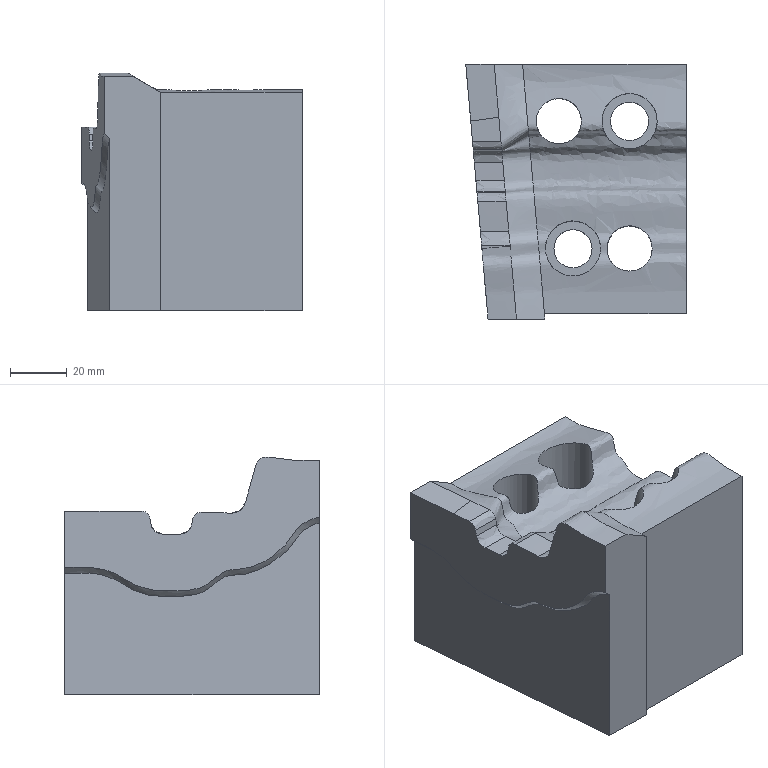Part | NX | features solid 2 | 1 solid | 32 faces | box 77.874 x 90 x 84.081 mm | volume 344852 mm3 | spline 16 | plane 10 | cylinder 6 | commonest cylinder face diameters 13.5 x2 16 x2 19.5 x2